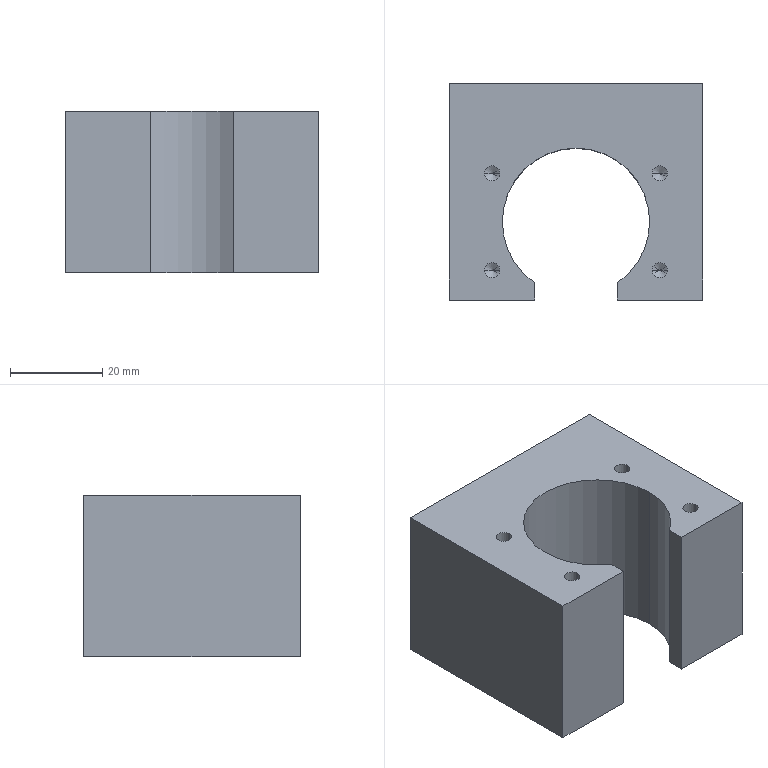Part | SolidWorks | features HoleWzd 2, 3DProfileFeature 1, Extrusion 1 | 1 solid | 52 faces | box 55 x 47 x 35 mm | volume 59809 mm3 | cone 24 | cylinder 19 | plane 9 | commonest cylinder face diameters 3.3 x8 5 x8 32 x3
STEP:
#1=CARTESIAN_POINT('',(-20.5,29.475,8.));
#2=VERTEX_POINT('',#1);
#3=CARTESIAN_POINT('',(-20.5,29.475,13.));
#4=VERTEX_POINT('',#3);
#5=CARTESIAN_POINT('',(-20.5,29.475,10.5));
#6=DIRECTION('',(0.,1.,0.));
#7=DIRECTION('',(0.,0.,1.));
#8=AXIS2_PLACEMENT_3D('',#5,#6,#7);
#9=CIRCLE('',#8,2.5);
#10=EDGE_CURVE('',#2,#4,#9,.T.);
#11=ORIENTED_EDGE('',*,*,#10,.F.);
#12=CARTESIAN_POINT('',(-20.5,30.,7.475));
#13=VERTEX_POINT('',#12);
#14=CARTESIAN_POINT('',(-20.5,30.,7.475));
#15=DIRECTION('',(0.,0.7071,-0.7071));
#16=VECTOR('',#15,1000.);
#17=LINE('',#14,#16);
#18=EDGE_CURVE('',#2,#13,#17,.T.);
#19=ORIENTED_EDGE('',*,*,#18,.T.);
#20=CARTESIAN_POINT('',(-20.5,30.,13.525));
#21=VERTEX_POINT('',#20);
#22=CARTESIAN_POINT('',(-20.5,30.,10.5));
#23=DIRECTION('',(0.,1.,0.));
#24=DIRECTION('',(0.,0.,1.));
#25=AXIS2_PLACEMENT_3D('',#22,#23,#24);
#26=CIRCLE('',#25,3.025);
#27=EDGE_CURVE('',#13,#21,#26,.T.);
#28=ORIENTED_EDGE('',*,*,#27,.T.);
#29=CARTESIAN_POINT('',(-20.5,30.,13.525));
#30=DIRECTION('',(0.,0.7071,0.7071));
#31=VECTOR('',#30,1000.);
#32=LINE('',#29,#31);
#33=EDGE_CURVE('',#4,#21,#32,.T.);
#34=ORIENTED_EDGE('',*,*,#33,.F.);
#35=EDGE_LOOP('',(#11,#19,#28,#34));
#36=FACE_OUTER_BOUND('',#35,.T.);
#37=CARTESIAN_POINT('',(-20.5,30.,10.5));
#38=DIRECTION('',(0.,1.,0.));
#39=DIRECTION('',(0.,0.,1.));
#40=AXIS2_PLACEMENT_3D('',#37,#38,#39);
#41=CONICAL_SURFACE('',#40,3.025,0.7854);
#42=ADVANCED_FACE('',(#36),#41,.F.);
#43=CARTESIAN_POINT('',(-20.5,18.,8.));
#44=VERTEX_POINT('',#43);
#45=CARTESIAN_POINT('',(-20.5,18.,13.));
#46=VERTEX_POINT('',#45);
#47=CARTESIAN_POINT('',(-20.5,18.,10.5));
#48=DIRECTION('',(0.,1.,0.));
#49=DIRECTION('',(0.,0.,1.));
#50=AXIS2_PLACEMENT_3D('',#47,#48,#49);
#51=CIRCLE('',#50,2.5);
#52=EDGE_CURVE('',#44,#46,#51,.T.);
#53=ORIENTED_EDGE('',*,*,#52,.F.);
#54=CARTESIAN_POINT('',(-20.5,30.,8.));
#55=DIRECTION('',(0.,1.,0.));
#56=VECTOR('',#55,1000.);
#57=LINE('',#54,#56);
#58=EDGE_CURVE('',#44,#2,#57,.T.);
#59=ORIENTED_EDGE('',*,*,#58,.T.);
#60=ORIENTED_EDGE('',*,*,#10,.T.);
#61=CARTESIAN_POINT('',(-20.5,30.,13.));
#62=DIRECTION('',(0.,1.,0.));
#63=VECTOR('',#62,1000.);
#64=LINE('',#61,#63);
#65=EDGE_CURVE('',#46,#4,#64,.T.);
#66=ORIENTED_EDGE('',*,*,#65,.F.);
#67=EDGE_LOOP('',(#53,#59,#60,#66));
#68=FACE_OUTER_BOUND('',#67,.T.);
#69=CARTESIAN_POINT('',(-20.5,30.,10.5));
#70=DIRECTION('',(0.,1.,0.));
#71=DIRECTION('',(0.,0.,1.));
#72=AXIS2_PLACEMENT_3D('',#69,#70,#71);
#73=CYLINDRICAL_SURFACE('',#72,2.5);
#74=ADVANCED_FACE('',(#68),#73,.F.);
#75=CARTESIAN_POINT('',(-20.5,16.498,10.5));
#76=VERTEX_POINT('',#75);
#77=CARTESIAN_POINT('',(-20.5,18.,13.));
#78=DIRECTION('',(0.,0.515,0.8572));
#79=VECTOR('',#78,1000.);
#80=LINE('',#77,#79);
#81=EDGE_CURVE('',#76,#46,#80,.T.);
#82=ORIENTED_EDGE('',*,*,#81,.F.);
#83=CARTESIAN_POINT('',(-20.5,18.,8.));
#84=DIRECTION('',(0.,0.515,-0.8572));
#85=VECTOR('',#84,1000.);
#86=LINE('',#83,#85);
#87=EDGE_CURVE('',#76,#44,#86,.T.);
#88=ORIENTED_EDGE('',*,*,#87,.T.);
#89=ORIENTED_EDGE('',*,*,#52,.T.);
#90=EDGE_LOOP('',(#82,#88,#89));
#91=FACE_OUTER_BOUND('',#90,.T.);
#92=CARTESIAN_POINT('',(-20.5,18.,10.5));
#93=DIRECTION('',(0.,1.,0.));
#94=DIRECTION('',(0.,0.,1.));
#95=AXIS2_PLACEMENT_3D('',#92,#93,#94);
#96=CONICAL_SURFACE('',#95,2.5,1.03);
#97=ADVANCED_FACE('',(#91),#96,.F.);
#98=CARTESIAN_POINT('',(-20.5,29.475,-13.));
#99=VERTEX_POINT('',#98);
#100=CARTESIAN_POINT('',(-20.5,29.475,-8.));
#101=VERTEX_POINT('',#100);
#102=CARTESIAN_POINT('',(-20.5,29.475,-10.5));
#103=DIRECTION('',(0.,1.,0.));
#104=DIRECTION('',(0.,0.,1.));
#105=AXIS2_PLACEMENT_3D('',#102,#103,#104);
#106=CIRCLE('',#105,2.5);
#107=EDGE_CURVE('',#99,#101,#106,.T.);
#108=ORIENTED_EDGE('',*,*,#107,.F.);
#109=CARTESIAN_POINT('',(-20.5,30.,-13.525));
#110=VERTEX_POINT('',#109);
#111=CARTESIAN_POINT('',(-20.5,30.,-13.525));
#112=DIRECTION('',(0.,0.7071,-0.7071));
#113=VECTOR('',#112,1000.);
#114=LINE('',#111,#113);
#115=EDGE_CURVE('',#99,#110,#114,.T.);
#116=ORIENTED_EDGE('',*,*,#115,.T.);
#117=CARTESIAN_POINT('',(-20.5,30.,-7.475));
#118=VERTEX_POINT('',#117);
#119=CARTESIAN_POINT('',(-20.5,30.,-10.5));
#120=DIRECTION('',(0.,1.,0.));
#121=DIRECTION('',(0.,0.,1.));
#122=AXIS2_PLACEMENT_3D('',#119,#120,#121);
#123=CIRCLE('',#122,3.025);
#124=EDGE_CURVE('',#110,#118,#123,.T.);
#125=ORIENTED_EDGE('',*,*,#124,.T.);
#126=CARTESIAN_POINT('',(-20.5,30.,-7.475));
#127=DIRECTION('',(0.,0.7071,0.7071));
#128=VECTOR('',#127,1000.);
#129=LINE('',#126,#128);
#130=EDGE_CURVE('',#101,#118,#129,.T.);
#131=ORIENTED_EDGE('',*,*,#130,.F.);
#132=EDGE_LOOP('',(#108,#116,#125,#131));
#133=FACE_OUTER_BOUND('',#132,.T.);
#134=CARTESIAN_POINT('',(-20.5,30.,-10.5));
#135=DIRECTION('',(0.,1.,0.));
#136=DIRECTION('',(0.,0.,1.));
#137=AXIS2_PLACEMENT_3D('',#134,#135,#136);
#138=CONICAL_SURFACE('',#137,3.025,0.7854);
#139=ADVANCED_FACE('',(#133),#138,.F.);
#140=CARTESIAN_POINT('',(-20.5,18.,-13.));
#141=VERTEX_POINT('',#140);
#142=CARTESIAN_POINT('',(-20.5,18.,-8.));
#143=VERTEX_POINT('',#142);
#144=CARTESIAN_POINT('',(-20.5,18.,-10.5));
#145=DIRECTION('',(0.,1.,0.));
#146=DIRECTION('',(0.,0.,1.));
#147=AXIS2_PLACEMENT_3D('',#144,#145,#146);
#148=CIRCLE('',#147,2.5);
#149=EDGE_CURVE('',#141,#143,#148,.T.);
#150=ORIENTED_EDGE('',*,*,#149,.F.);
#151=CARTESIAN_POINT('',(-20.5,30.,-13.));
#152=DIRECTION('',(0.,1.,0.));
#153=VECTOR('',#152,1000.);
#154=LINE('',#151,#153);
#155=EDGE_CURVE('',#141,#99,#154,.T.);
#156=ORIENTED_EDGE('',*,*,#155,.T.);
#157=ORIENTED_EDGE('',*,*,#107,.T.);
#158=CARTESIAN_POINT('',(-20.5,30.,-8.));
#159=DIRECTION('',(0.,1.,0.));
#160=VECTOR('',#159,1000.);
#161=LINE('',#158,#160);
#162=EDGE_CURVE('',#143,#101,#161,.T.);
#163=ORIENTED_EDGE('',*,*,#162,.F.);
#164=EDGE_LOOP('',(#150,#156,#157,#163));
#165=FACE_OUTER_BOUND('',#164,.T.);
#166=CARTESIAN_POINT('',(-20.5,30.,-10.5));
#167=DIRECTION('',(0.,1.,0.));
#168=DIRECTION('',(0.,0.,1.));
#169=AXIS2_PLACEMENT_3D('',#166,#167,#168);
#170=CYLINDRICAL_SURFACE('',#169,2.5);
#171=ADVANCED_FACE('',(#165),#170,.F.);
#172=CARTESIAN_POINT('',(-20.5,16.498,-10.5));
#173=VERTEX_POINT('',#172);
#174=CARTESIAN_POINT('',(-20.5,18.,-8.));
#175=DIRECTION('',(0.,0.515,0.8572));
#176=VECTOR('',#175,1000.);
#177=LINE('',#174,#176);
#178=EDGE_CURVE('',#173,#143,#177,.T.);
#179=ORIENTED_EDGE('',*,*,#178,.F.);
#180=CARTESIAN_POINT('',(-20.5,18.,-13.));
#181=DIRECTION('',(0.,0.515,-0.8572));
#182=VECTOR('',#181,1000.);
#183=LINE('',#180,#182);
#184=EDGE_CURVE('',#173,#141,#183,.T.);
#185=ORIENTED_EDGE('',*,*,#184,.T.);
#186=ORIENTED_EDGE('',*,*,#149,.T.);
#187=EDGE_LOOP('',(#179,#185,#186));
#188=FACE_OUTER_BOUND('',#187,.T.);
#189=CARTESIAN_POINT('',(-20.5,18.,-10.5));
#190=DIRECTION('',(0.,1.,0.));
#191=DIRECTION('',(0.,0.,1.));
#192=AXIS2_PLACEMENT_3D('',#189,#190,#191);
#193=CONICAL_SURFACE('',#192,2.5,1.03);
#194=ADVANCED_FACE('',(#188),#193,.F.);
#195=CARTESIAN_POINT('',(20.5,29.475,-13.));
#196=VERTEX_POINT('',#195);
#197=CARTESIAN_POINT('',(20.5,29.475,-8.));
#198=VERTEX_POINT('',#197);
#199=CARTESIAN_POINT('',(20.5,29.475,-10.5));
#200=DIRECTION('',(0.,1.,0.));
#201=DIRECTION('',(0.,0.,1.));
#202=AXIS2_PLACEMENT_3D('',#199,#200,#201);
#203=CIRCLE('',#202,2.5);
#204=EDGE_CURVE('',#196,#198,#203,.T.);
#205=ORIENTED_EDGE('',*,*,#204,.F.);
#206=CARTESIAN_POINT('',(20.5,30.,-13.525));
#207=VERTEX_POINT('',#206);
#208=CARTESIAN_POINT('',(20.5,30.,-13.525));
#209=DIRECTION('',(0.,0.7071,-0.7071));
#210=VECTOR('',#209,1000.);
#211=LINE('',#208,#210);
#212=EDGE_CURVE('',#196,#207,#211,.T.);
#213=ORIENTED_EDGE('',*,*,#212,.T.);
#214=CARTESIAN_POINT('',(20.5,30.,-7.475));
#215=VERTEX_POINT('',#214);
#216=CARTESIAN_POINT('',(20.5,30.,-10.5));
#217=DIRECTION('',(0.,1.,0.));
#218=DIRECTION('',(0.,0.,1.));
#219=AXIS2_PLACEMENT_3D('',#216,#217,#218);
#220=CIRCLE('',#219,3.025);
#221=EDGE_CURVE('',#207,#215,#220,.T.);
#222=ORIENTED_EDGE('',*,*,#221,.T.);
#223=CARTESIAN_POINT('',(20.5,30.,-7.475));
#224=DIRECTION('',(0.,0.7071,0.7071));
#225=VECTOR('',#224,1000.);
#226=LINE('',#223,#225);
#227=EDGE_CURVE('',#198,#215,#226,.T.);
#228=ORIENTED_EDGE('',*,*,#227,.F.);
#229=EDGE_LOOP('',(#205,#213,#222,#228));
#230=FACE_OUTER_BOUND('',#229,.T.);
#231=CARTESIAN_POINT('',(20.5,30.,-10.5));
#232=DIRECTION('',(0.,1.,0.));
#233=DIRECTION('',(0.,0.,1.));
#234=AXIS2_PLACEMENT_3D('',#231,#232,#233);
#235=CONICAL_SURFACE('',#234,3.025,0.7854);
#236=ADVANCED_FACE('',(#230),#235,.F.);
#237=CARTESIAN_POINT('',(20.5,18.,-13.));
#238=VERTEX_POINT('',#237);
#239=CARTESIAN_POINT('',(20.5,18.,-8.));
#240=VERTEX_POINT('',#239);
#241=CARTESIAN_POINT('',(20.5,18.,-10.5));
#242=DIRECTION('',(0.,1.,0.));
#243=DIRECTION('',(0.,0.,1.));
#244=AXIS2_PLACEMENT_3D('',#241,#242,#243);
#245=CIRCLE('',#244,2.5);
#246=EDGE_CURVE('',#238,#240,#245,.T.);
#247=ORIENTED_EDGE('',*,*,#246,.F.);
#248=CARTESIAN_POINT('',(20.5,30.,-13.));
#249=DIRECTION('',(0.,1.,0.));
#250=VECTOR('',#249,1000.);
#251=LINE('',#248,#250);
#252=EDGE_CURVE('',#238,#196,#251,.T.);
#253=ORIENTED_EDGE('',*,*,#252,.T.);
#254=ORIENTED_EDGE('',*,*,#204,.T.);
#255=CARTESIAN_POINT('',(20.5,30.,-8.));
#256=DIRECTION('',(0.,1.,0.));
#257=VECTOR('',#256,1000.);
#258=LINE('',#255,#257);
#259=EDGE_CURVE('',#240,#198,#258,.T.);
#260=ORIENTED_EDGE('',*,*,#259,.F.);
#261=EDGE_LOOP('',(#247,#253,#254,#260));
#262=FACE_OUTER_BOUND('',#261,.T.);
#263=CARTESIAN_POINT('',(20.5,30.,-10.5));
#264=DIRECTION('',(0.,1.,0.));
#265=DIRECTION('',(0.,0.,1.));
#266=AXIS2_PLACEMENT_3D('',#263,#264,#265);
#267=CYLINDRICAL_SURFACE('',#266,2.5);
#268=ADVANCED_FACE('',(#262),#267,.F.);
#269=CARTESIAN_POINT('',(20.5,16.498,-10.5));
#270=VERTEX_POINT('',#269);
#271=CARTESIAN_POINT('',(20.5,18.,-8.));
#272=DIRECTION('',(0.,0.515,0.8572));
#273=VECTOR('',#272,1000.);
#274=LINE('',#271,#273);
#275=EDGE_CURVE('',#270,#240,#274,.T.);
#276=ORIENTED_EDGE('',*,*,#275,.F.);
#277=CARTESIAN_POINT('',(20.5,18.,-13.));
#278=DIRECTION('',(0.,0.515,-0.8572));
#279=VECTOR('',#278,1000.);
#280=LINE('',#277,#279);
#281=EDGE_CURVE('',#270,#238,#280,.T.);
#282=ORIENTED_EDGE('',*,*,#281,.T.);
#283=ORIENTED_EDGE('',*,*,#246,.T.);
#284=EDGE_LOOP('',(#276,#282,#283));
#285=FACE_OUTER_BOUND('',#284,.T.);
#286=CARTESIAN_POINT('',(20.5,18.,-10.5));
#287=DIRECTION('',(0.,1.,0.));
#288=DIRECTION('',(0.,0.,1.));
#289=AXIS2_PLACEMENT_3D('',#286,#287,#288);
#290=CONICAL_SURFACE('',#289,2.5,1.03);
#291=ADVANCED_FACE('',(#285),#290,.F.);
#292=CARTESIAN_POINT('',(20.5,29.475,8.));
#293=VERTEX_POINT('',#292);
#294=CARTESIAN_POINT('',(20.5,29.475,13.));
#295=VERTEX_POINT('',#294);
#296=CARTESIAN_POINT('',(20.5,29.475,10.5));
#297=DIRECTION('',(0.,1.,0.));
#298=DIRECTION('',(0.,0.,1.));
#299=AXIS2_PLACEMENT_3D('',#296,#297,#298);
#300=CIRCLE('',#299,2.5);
#301=EDGE_CURVE('',#293,#295,#300,.T.);
#302=ORIENTED_EDGE('',*,*,#301,.F.);
#303=CARTESIAN_POINT('',(20.5,30.,7.475));
#304=VERTEX_POINT('',#303);
#305=CARTESIAN_POINT('',(20.5,30.,7.475));
#306=DIRECTION('',(0.,0.7071,-0.7071));
#307=VECTOR('',#306,1000.);
#308=LINE('',#305,#307);
#309=EDGE_CURVE('',#293,#304,#308,.T.);
#310=ORIENTED_EDGE('',*,*,#309,.T.);
#311=CARTESIAN_POINT('',(20.5,30.,13.525));
#312=VERTEX_POINT('',#311);
#313=CARTESIAN_POINT('',(20.5,30.,10.5));
#314=DIRECTION('',(0.,1.,0.));
#315=DIRECTION('',(0.,0.,1.));
#316=AXIS2_PLACEMENT_3D('',#313,#314,#315);
#317=CIRCLE('',#316,3.025);
#318=EDGE_CURVE('',#304,#312,#317,.T.);
#319=ORIENTED_EDGE('',*,*,#318,.T.);
#320=CARTESIAN_POINT('',(20.5,30.,13.525));
#321=DIRECTION('',(0.,0.7071,0.7071));
#322=VECTOR('',#321,1000.);
#323=LINE('',#320,#322);
#324=EDGE_CURVE('',#295,#312,#323,.T.);
#325=ORIENTED_EDGE('',*,*,#324,.F.);
#326=EDGE_LOOP('',(#302,#310,#319,#325));
#327=FACE_OUTER_BOUND('',#326,.T.);
#328=CARTESIAN_POINT('',(20.5,30.,10.5));
#329=DIRECTION('',(0.,1.,0.));
#330=DIRECTION('',(0.,0.,1.));
#331=AXIS2_PLACEMENT_3D('',#328,#329,#330);
#332=CONICAL_SURFACE('',#331,3.025,0.7854);
#333=ADVANCED_FACE('',(#327),#332,.F.);
#334=CARTESIAN_POINT('',(20.5,18.,8.));
#335=VERTEX_POINT('',#334);
#336=CARTESIAN_POINT('',(20.5,18.,13.));
#337=VERTEX_POINT('',#336);
#338=CARTESIAN_POINT('',(20.5,18.,10.5));
#339=DIRECTION('',(0.,1.,0.));
#340=DIRECTION('',(0.,0.,1.));
#341=AXIS2_PLACEMENT_3D('',#338,#339,#340);
#342=CIRCLE('',#341,2.5);
#343=EDGE_CURVE('',#335,#337,#342,.T.);
#344=ORIENTED_EDGE('',*,*,#343,.F.);
#345=CARTESIAN_POINT('',(20.5,30.,8.));
#346=DIRECTION('',(0.,1.,0.));
#347=VECTOR('',#346,1000.);
#348=LINE('',#345,#347);
#349=EDGE_CURVE('',#335,#293,#348,.T.);
#350=ORIENTED_EDGE('',*,*,#349,.T.);
#351=ORIENTED_EDGE('',*,*,#301,.T.);
#352=CARTESIAN_POINT('',(20.5,30.,13.));
#353=DIRECTION('',(0.,1.,0.));
#354=VECTOR('',#353,1000.);
#355=LINE('',#352,#354);
#356=EDGE_CURVE('',#337,#295,#355,.T.);
#357=ORIENTED_EDGE('',*,*,#356,.F.);
#358=EDGE_LOOP('',(#344,#350,#351,#357));
#359=FACE_OUTER_BOUND('',#358,.T.);
#360=CARTESIAN_POINT('',(20.5,30.,10.5));
#361=DIRECTION('',(0.,1.,0.));
#362=DIRECTION('',(0.,0.,1.));
#363=AXIS2_PLACEMENT_3D('',#360,#361,#362);
#364=CYLINDRICAL_SURFACE('',#363,2.5);
#365=ADVANCED_FACE('',(#359),#364,.F.);
#366=CARTESIAN_POINT('',(20.5,16.498,10.5));
#367=VERTEX_POINT('',#366);
#368=CARTESIAN_POINT('',(20.5,18.,13.));
#369=DIRECTION('',(0.,0.515,0.8572));
#370=VECTOR('',#369,1000.);
#371=LINE('',#368,#370);
#372=EDGE_CURVE('',#367,#337,#371,.T.);
#373=ORIENTED_EDGE('',*,*,#372,.F.);
#374=CARTESIAN_POINT('',(20.5,18.,8.));
#375=DIRECTION('',(0.,0.515,-0.8572));
#376=VECTOR('',#375,1000.);
#377=LINE('',#374,#376);
#378=EDGE_CURVE('',#367,#335,#377,.T.);
#379=ORIENTED_EDGE('',*,*,#378,.T.);
#380=ORIENTED_EDGE('',*,*,#343,.T.);
#381=EDGE_LOOP('',(#373,#379,#380));
#382=FACE_OUTER_BOUND('',#381,.T.);
#383=CARTESIAN_POINT('',(20.5,18.,10.5));
#384=DIRECTION('',(0.,1.,0.));
#385=DIRECTION('',(0.,0.,1.));
#386=AXIS2_PLACEMENT_3D('',#383,#384,#385);
#387=CONICAL_SURFACE('',#386,2.5,1.03);
#388=ADVANCED_FACE('',(#382),#387,.F.);
#389=CARTESIAN_POINT('',(16.537,10.5,8.));
#390=VERTEX_POINT('',#389);
#391=CARTESIAN_POINT('',(19.837,10.5,8.));
#392=VERTEX_POINT('',#391);
#393=CARTESIAN_POINT('',(18.187,10.5,8.));
#394=DIRECTION('',(0.,0.,1.));
#395=DIRECTION('',(1.,0.,0.));
#396=AXIS2_PLACEMENT_3D('',#393,#394,#395);
#397=CIRCLE('',#396,1.65);
#398=EDGE_CURVE('',#390,#392,#397,.T.);
#399=ORIENTED_EDGE('',*,*,#398,.F.);
#400=CARTESIAN_POINT('',(16.537,10.5,17.5));
#401=VERTEX_POINT('',#400);
#402=CARTESIAN_POINT('',(16.537,10.5,17.5));
#403=DIRECTION('',(0.,0.,1.));
#404=VECTOR('',#403,1000.);
#405=LINE('',#402,#404);
#406=EDGE_CURVE('',#390,#401,#405,.T.);
#407=ORIENTED_EDGE('',*,*,#406,.T.);
#408=CARTESIAN_POINT('',(19.837,10.5,17.5));
#409=VERTEX_POINT('',#408);
#410=CARTESIAN_POINT('',(18.187,10.5,17.5));
#411=DIRECTION('',(0.,0.,1.));
#412=DIRECTION('',(1.,0.,0.));
#413=AXIS2_PLACEMENT_3D('',#410,#411,#412);
#414=CIRCLE('',#413,1.65);
#415=EDGE_CURVE('',#401,#409,#414,.T.);
#416=ORIENTED_EDGE('',*,*,#415,.T.);
#417=CARTESIAN_POINT('',(19.837,10.5,17.5));
#418=DIRECTION('',(0.,0.,1.));
#419=VECTOR('',#418,1000.);
#420=LINE('',#417,#419);
#421=EDGE_CURVE('',#392,#409,#420,.T.);
#422=ORIENTED_EDGE('',*,*,#421,.F.);
#423=EDGE_LOOP('',(#399,#407,#416,#422));
#424=FACE_OUTER_BOUND('',#423,.T.);
#425=CARTESIAN_POINT('',(18.187,10.5,17.5));
#426=DIRECTION('',(0.,0.,1.));
#427=DIRECTION('',(1.,0.,0.));
#428=AXIS2_PLACEMENT_3D('',#425,#426,#427);
#429=CYLINDRICAL_SURFACE('',#428,1.65);
#430=ADVANCED_FACE('',(#424),#429,.F.);
#431=CARTESIAN_POINT('',(18.187,10.5,7.009));
#432=VERTEX_POINT('',#431);
#433=CARTESIAN_POINT('',(19.837,10.5,8.));
#434=DIRECTION('',(0.8572,0.,0.515));
#435=VECTOR('',#434,1000.);
#436=LINE('',#433,#435);
#437=EDGE_CURVE('',#432,#392,#436,.T.);
#438=ORIENTED_EDGE('',*,*,#437,.F.);
#439=CARTESIAN_POINT('',(16.537,10.5,8.));
#440=DIRECTION('',(-0.8572,0.,0.515));
#441=VECTOR('',#440,1000.);
#442=LINE('',#439,#441);
#443=EDGE_CURVE('',#432,#390,#442,.T.);
#444=ORIENTED_EDGE('',*,*,#443,.T.);
#445=ORIENTED_EDGE('',*,*,#398,.T.);
#446=EDGE_LOOP('',(#438,#444,#445));
#447=FACE_OUTER_BOUND('',#446,.T.);
#448=CARTESIAN_POINT('',(18.187,10.5,8.));
#449=DIRECTION('',(0.,0.,1.));
#450=DIRECTION('',(1.,0.,0.));
#451=AXIS2_PLACEMENT_3D('',#448,#449,#450);
#452=CONICAL_SURFACE('',#451,1.65,1.03);
#453=ADVANCED_FACE('',(#447),#452,.F.);
#454=CARTESIAN_POINT('',(16.537,-10.5,8.));
#455=VERTEX_POINT('',#454);
#456=CARTESIAN_POINT('',(19.837,-10.5,8.));
#457=VERTEX_POINT('',#456);
#458=CARTESIAN_POINT('',(18.187,-10.5,8.));
#459=DIRECTION('',(0.,0.,1.));
#460=DIRECTION('',(1.,0.,0.));
#461=AXIS2_PLACEMENT_3D('',#458,#459,#460);
#462=CIRCLE('',#461,1.65);
#463=EDGE_CURVE('',#455,#457,#462,.T.);
#464=ORIENTED_EDGE('',*,*,#463,.F.);
#465=CARTESIAN_POINT('',(16.537,-10.5,17.5));
#466=VERTEX_POINT('',#465);
#467=CARTESIAN_POINT('',(16.537,-10.5,17.5));
#468=DIRECTION('',(0.,0.,1.));
#469=VECTOR('',#468,1000.);
#470=LINE('',#467,#469);
#471=EDGE_CURVE('',#455,#466,#470,.T.);
#472=ORIENTED_EDGE('',*,*,#471,.T.);
#473=CARTESIAN_POINT('',(19.837,-10.5,17.5));
#474=VERTEX_POINT('',#473);
#475=CARTESIAN_POINT('',(18.187,-10.5,17.5));
#476=DIRECTION('',(0.,0.,1.));
#477=DIRECTION('',(1.,0.,0.));
#478=AXIS2_PLACEMENT_3D('',#475,#476,#477);
#479=CIRCLE('',#478,1.65);
#480=EDGE_CURVE('',#466,#474,#479,.T.);
#481=ORIENTED_EDGE('',*,*,#480,.T.);
#482=CARTESIAN_POINT('',(19.837,-10.5,17.5));
#483=DIRECTION('',(0.,0.,1.));
#484=VECTOR('',#483,1000.);
#485=LINE('',#482,#484);
#486=EDGE_CURVE('',#457,#474,#485,.T.);
#487=ORIENTED_EDGE('',*,*,#486,.F.);
#488=EDGE_LOOP('',(#464,#472,#481,#487));
#489=FACE_OUTER_BOUND('',#488,.T.);
#490=CARTESIAN_POINT('',(18.187,-10.5,17.5));
#491=DIRECTION('',(0.,0.,1.));
#492=DIRECTION('',(1.,0.,0.));
#493=AXIS2_PLACEMENT_3D('',#490,#491,#492);
#494=CYLINDRICAL_SURFACE('',#493,1.65);
#495=ADVANCED_FACE('',(#489),#494,.F.);
#496=CARTESIAN_POINT('',(18.187,-10.5,7.009));
#497=VERTEX_POINT('',#496);
#498=CARTESIAN_POINT('',(19.837,-10.5,8.));
#499=DIRECTION('',(0.8572,0.,0.515));
#500=VECTOR('',#499,1000.);
#501=LINE('',#498,#500);
#502=EDGE_CURVE('',#497,#457,#501,.T.);
#503=ORIENTED_EDGE('',*,*,#502,.F.);
#504=CARTESIAN_POINT('',(16.537,-10.5,8.));
#505=DIRECTION('',(-0.8572,0.,0.515));
#506=VECTOR('',#505,1000.);
#507=LINE('',#504,#506);
#508=EDGE_CURVE('',#497,#455,#507,.T.);
#509=ORIENTED_EDGE('',*,*,#508,.T.);
#510=ORIENTED_EDGE('',*,*,#463,.T.);
#511=EDGE_LOOP('',(#503,#509,#510));
#512=FACE_OUTER_BOUND('',#511,.T.);
#513=CARTESIAN_POINT('',(18.187,-10.5,8.));
#514=DIRECTION('',(0.,0.,1.));
#515=DIRECTION('',(1.,0.,0.));
#516=AXIS2_PLACEMENT_3D('',#513,#514,#515);
#517=CONICAL_SURFACE('',#516,1.65,1.03);
#518=ADVANCED_FACE('',(#512),#517,.F.);
#519=CARTESIAN_POINT('',(-19.837,-10.5,8.));
#520=VERTEX_POINT('',#519);
#521=CARTESIAN_POINT('',(-16.537,-10.5,8.));
#522=VERTEX_POINT('',#521);
#523=CARTESIAN_POINT('',(-18.187,-10.5,8.));
#524=DIRECTION('',(0.,0.,1.));
#525=DIRECTION('',(1.,0.,0.));
#526=AXIS2_PLACEMENT_3D('',#523,#524,#525);
#527=CIRCLE('',#526,1.65);
#528=EDGE_CURVE('',#520,#522,#527,.T.);
#529=ORIENTED_EDGE('',*,*,#528,.F.);
#530=CARTESIAN_POINT('',(-19.837,-10.5,17.5));
#531=VERTEX_POINT('',#530);
#532=CARTESIAN_POINT('',(-19.837,-10.5,17.5));
#533=DIRECTION('',(0.,0.,1.));
#534=VECTOR('',#533,1000.);
#535=LINE('',#532,#534);
#536=EDGE_CURVE('',#520,#531,#535,.T.);
#537=ORIENTED_EDGE('',*,*,#536,.T.);
#538=CARTESIAN_POINT('',(-16.537,-10.5,17.5));
#539=VERTEX_POINT('',#538);
#540=CARTESIAN_POINT('',(-18.187,-10.5,17.5));
#541=DIRECTION('',(0.,0.,1.));
#542=DIRECTION('',(1.,0.,0.));
#543=AXIS2_PLACEMENT_3D('',#540,#541,#542);
#544=CIRCLE('',#543,1.65);
#545=EDGE_CURVE('',#531,#539,#544,.T.);
#546=ORIENTED_EDGE('',*,*,#545,.T.);
#547=CARTESIAN_POINT('',(-16.537,-10.5,17.5));
#548=DIRECTION('',(0.,0.,1.));
#549=VECTOR('',#548,1000.);
#550=LINE('',#547,#549);
#551=EDGE_CURVE('',#522,#539,#550,.T.);
#552=ORIENTED_EDGE('',*,*,#551,.F.);
#553=EDGE_LOOP('',(#529,#537,#546,#552));
#554=FACE_OUTER_BOUND('',#553,.T.);
#555=CARTESIAN_POINT('',(-18.187,-10.5,17.5));
#556=DIRECTION('',(0.,0.,1.));
#557=DIRECTION('',(1.,0.,0.));
#558=AXIS2_PLACEMENT_3D('',#555,#556,#557);
#559=CYLINDRICAL_SURFACE('',#558,1.65);
#560=ADVANCED_FACE('',(#554),#559,.F.);
#561=CARTESIAN_POINT('',(-18.187,-10.5,7.009));
#562=VERTEX_POINT('',#561);
#563=CARTESIAN_POINT('',(-16.537,-10.5,8.));
#564=DIRECTION('',(0.8572,0.,0.515));
#565=VECTOR('',#564,1000.);
#566=LINE('',#563,#565);
#567=EDGE_CURVE('',#562,#522,#566,.T.);
#568=ORIENTED_EDGE('',*,*,#567,.F.);
#569=CARTESIAN_POINT('',(-19.837,-10.5,8.));
#570=DIRECTION('',(-0.8572,0.,0.515));
#571=VECTOR('',#570,1000.);
#572=LINE('',#569,#571);
#573=EDGE_CURVE('',#562,#520,#572,.T.);
#574=ORIENTED_EDGE('',*,*,#573,.T.);
#575=ORIENTED_EDGE('',*,*,#528,.T.);
#576=EDGE_LOOP('',(#568,#574,#575));
#577=FACE_OUTER_BOUND('',#576,.T.);
#578=CARTESIAN_POINT('',(-18.187,-10.5,8.));
#579=DIRECTION('',(0.,0.,1.));
#580=DIRECTION('',(1.,0.,0.));
#581=AXIS2_PLACEMENT_3D('',#578,#579,#580);
#582=CONICAL_SURFACE('',#581,1.65,1.03);
#583=ADVANCED_FACE('',(#577),#582,.F.);
#584=CARTESIAN_POINT('',(-19.837,10.5,8.));
#585=VERTEX_POINT('',#584);
#586=CARTESIAN_POINT('',(-16.537,10.5,8.));
#587=VERTEX_POINT('',#586);
#588=CARTESIAN_POINT('',(-18.187,10.5,8.));
#589=DIRECTION('',(0.,0.,1.));
#590=DIRECTION('',(1.,0.,0.));
#591=AXIS2_PLACEMENT_3D('',#588,#589,#590);
#592=CIRCLE('',#591,1.65);
#593=EDGE_CURVE('',#585,#587,#592,.T.);
#594=ORIENTED_EDGE('',*,*,#593,.F.);
#595=CARTESIAN_POINT('',(-19.837,10.5,17.5));
#596=VERTEX_POINT('',#595);
#597=CARTESIAN_POINT('',(-19.837,10.5,17.5));
#598=DIRECTION('',(0.,0.,1.));
#599=VECTOR('',#598,1000.);
#600=LINE('',#597,#599);
#601=EDGE_CURVE('',#585,#596,#600,.T.);
#602=ORIENTED_EDGE('',*,*,#601,.T.);
#603=CARTESIAN_POINT('',(-16.537,10.5,17.5));
#604=VERTEX_POINT('',#603);
#605=CARTESIAN_POINT('',(-18.187,10.5,17.5));
#606=DIRECTION('',(0.,0.,1.));
#607=DIRECTION('',(1.,0.,0.));
#608=AXIS2_PLACEMENT_3D('',#605,#606,#607);
#609=CIRCLE('',#608,1.65);
#610=EDGE_CURVE('',#596,#604,#609,.T.);
#611=ORIENTED_EDGE('',*,*,#610,.T.);
#612=CARTESIAN_POINT('',(-16.537,10.5,17.5));
#613=DIRECTION('',(0.,0.,1.));
#614=VECTOR('',#613,1000.);
#615=LINE('',#612,#614);
#616=EDGE_CURVE('',#587,#604,#615,.T.);
#617=ORIENTED_EDGE('',*,*,#616,.F.);
#618=EDGE_LOOP('',(#594,#602,#611,#617));
#619=FACE_OUTER_BOUND('',#618,.T.);
#620=CARTESIAN_POINT('',(-18.187,10.5,17.5));
#621=DIRECTION('',(0.,0.,1.));
#622=DIRECTION('',(1.,0.,0.));
#623=AXIS2_PLACEMENT_3D('',#620,#621,#622);
#624=CYLINDRICAL_SURFACE('',#623,1.65);
#625=ADVANCED_FACE('',(#619),#624,.F.);
#626=CARTESIAN_POINT('',(-18.187,10.5,7.009));
#627=VERTEX_POINT('',#626);
#628=CARTESIAN_POINT('',(-16.537,10.5,8.));
#629=DIRECTION('',(0.8572,0.,0.515));
#630=VECTOR('',#629,1000.);
#631=LINE('',#628,#630);
#632=EDGE_CURVE('',#627,#587,#631,.T.);
#633=ORIENTED_EDGE('',*,*,#632,.F.);
#634=CARTESIAN_POINT('',(-19.837,10.5,8.));
#635=DIRECTION('',(-0.8572,0.,0.515));
#636=VECTOR('',#635,1000.);
#637=LINE('',#634,#636);
#638=EDGE_CURVE('',#627,#585,#637,.T.);
#639=ORIENTED_EDGE('',*,*,#638,.T.);
#640=ORIENTED_EDGE('',*,*,#593,.T.);
#641=EDGE_LOOP('',(#633,#639,#640));
#642=FACE_OUTER_BOUND('',#641,.T.);
#643=CARTESIAN_POINT('',(-18.187,10.5,8.));
#644=DIRECTION('',(0.,0.,1.));
#645=DIRECTION('',(1.,0.,0.));
#646=AXIS2_PLACEMENT_3D('',#643,#644,#645);
#647=CONICAL_SURFACE('',#646,1.65,1.03);
#648=ADVANCED_FACE('',(#642),#647,.F.);
#649=CARTESIAN_POINT('',(16.,0.,17.5));
#650=VERTEX_POINT('',#649);
#651=CARTESIAN_POINT('',(9.,-13.229,17.5));
#652=VERTEX_POINT('',#651);
#653=CARTESIAN_POINT('',(0.,0.,17.5));
#654=DIRECTION('',(0.,0.,-1.));
#655=DIRECTION('',(1.,0.,0.));
#656=AXIS2_PLACEMENT_3D('',#653,#654,#655);
#657=CIRCLE('',#656,16.);
#658=EDGE_CURVE('',#650,#652,#657,.T.);
#659=ORIENTED_EDGE('',*,*,#658,.F.);
#660=CARTESIAN_POINT('',(16.,0.,-17.5));
#661=VERTEX_POINT('',#660);
#662=CARTESIAN_POINT('',(16.,0.,17.5));
#663=DIRECTION('',(0.,0.,-1.));
#664=VECTOR('',#663,1000.);
#665=LINE('',#662,#664);
#666=EDGE_CURVE('',#650,#661,#665,.T.);
#667=ORIENTED_EDGE('',*,*,#666,.T.);
#668=CARTESIAN_POINT('',(9.,-13.229,-17.5));
#669=VERTEX_POINT('',#668);
#670=CARTESIAN_POINT('',(0.,0.,-17.5));
#671=DIRECTION('',(0.,0.,-1.));
#672=DIRECTION('',(1.,0.,0.));
#673=AXIS2_PLACEMENT_3D('',#670,#671,#672);
#674=CIRCLE('',#673,16.);
#675=EDGE_CURVE('',#661,#669,#674,.T.);
#676=ORIENTED_EDGE('',*,*,#675,.T.);
#677=CARTESIAN_POINT('',(9.,-13.229,17.5));
#678=DIRECTION('',(0.,0.,-1.));
#679=VECTOR('',#678,1000.);
#680=LINE('',#677,#679);
#681=EDGE_CURVE('',#652,#669,#680,.T.);
#682=ORIENTED_EDGE('',*,*,#681,.F.);
#683=EDGE_LOOP('',(#659,#667,#676,#682));
#684=FACE_OUTER_BOUND('',#683,.T.);
#685=CARTESIAN_POINT('',(0.,0.,17.5));
#686=DIRECTION('',(0.,0.,-1.));
#687=DIRECTION('',(-1.,0.,0.));
#688=AXIS2_PLACEMENT_3D('',#685,#686,#687);
#689=CYLINDRICAL_SURFACE('',#688,16.);
#690=ADVANCED_FACE('',(#684),#689,.F.);
#691=ORIENTED_EDGE('',*,*,#666,.F.);
#692=CARTESIAN_POINT('',(-16.,0.,17.5));
#693=VERTEX_POINT('',#692);
#694=CARTESIAN_POINT('',(0.,0.,17.5));
#695=DIRECTION('',(0.,0.,-1.));
#696=DIRECTION('',(1.,0.,0.));
#697=AXIS2_PLACEMENT_3D('',#694,#695,#696);
#698=CIRCLE('',#697,16.);
#699=EDGE_CURVE('',#693,#650,#698,.T.);
#700=ORIENTED_EDGE('',*,*,#699,.F.);
#701=CARTESIAN_POINT('',(-16.,0.,-17.5));
#702=VERTEX_POINT('',#701);
#703=CARTESIAN_POINT('',(-16.,0.,17.5));
#704=DIRECTION('',(0.,0.,-1.));
#705=VECTOR('',#704,1000.);
#706=LINE('',#703,#705);
#707=EDGE_CURVE('',#693,#702,#706,.T.);
#708=ORIENTED_EDGE('',*,*,#707,.T.);
#709=CARTESIAN_POINT('',(0.,0.,-17.5));
#710=DIRECTION('',(0.,0.,-1.));
#711=DIRECTION('',(1.,0.,0.));
#712=AXIS2_PLACEMENT_3D('',#709,#710,#711);
#713=CIRCLE('',#712,16.);
#714=EDGE_CURVE('',#702,#661,#713,.T.);
#715=ORIENTED_EDGE('',*,*,#714,.T.);
#716=EDGE_LOOP('',(#691,#700,#708,#715));
#717=FACE_OUTER_BOUND('',#716,.T.);
#718=CARTESIAN_POINT('',(0.,0.,17.5));
#719=DIRECTION('',(0.,0.,-1.));
#720=DIRECTION('',(-1.,0.,0.));
#721=AXIS2_PLACEMENT_3D('',#718,#719,#720);
#722=CYLINDRICAL_SURFACE('',#721,16.);
#723=ADVANCED_FACE('',(#717),#722,.F.);
#724=CARTESIAN_POINT('',(-27.5,30.,-17.5));
#725=VERTEX_POINT('',#724);
#726=CARTESIAN_POINT('',(-27.5,-17.,-17.5));
#727=VERTEX_POINT('',#726);
#728=CARTESIAN_POINT('',(-27.5,30.,-17.5));
#729=DIRECTION('',(0.,-1.,0.));
#730=VECTOR('',#729,1000.);
#731=LINE('',#728,#730);
#732=EDGE_CURVE('',#725,#727,#731,.T.);
#733=ORIENTED_EDGE('',*,*,#732,.T.);
#734=CARTESIAN_POINT('',(-27.5,-17.,17.5));
#735=VERTEX_POINT('',#734);
#736=CARTESIAN_POINT('',(-27.5,-17.,17.5));
#737=DIRECTION('',(0.,0.,-1.));
#738=VECTOR('',#737,1000.);
#739=LINE('',#736,#738);
#740=EDGE_CURVE('',#735,#727,#739,.T.);
#741=ORIENTED_EDGE('',*,*,#740,.F.);
#742=CARTESIAN_POINT('',(-27.5,30.,17.5));
#743=VERTEX_POINT('',#742);
#744=CARTESIAN_POINT('',(-27.5,30.,17.5));
#745=DIRECTION('',(0.,-1.,0.));
#746=VECTOR('',#745,1000.);
#747=LINE('',#744,#746);
#748=EDGE_CURVE('',#743,#735,#747,.T.);
#749=ORIENTED_EDGE('',*,*,#748,.F.);
#750=CARTESIAN_POINT('',(-27.5,30.,17.5));
#751=DIRECTION('',(0.,0.,-1.));
#752=VECTOR('',#751,1000.);
#753=LINE('',#750,#752);
#754=EDGE_CURVE('',#743,#725,#753,.T.);
#755=ORIENTED_EDGE('',*,*,#754,.T.);
#756=EDGE_LOOP('',(#733,#741,#749,#755));
#757=FACE_OUTER_BOUND('',#756,.T.);
#758=CARTESIAN_POINT('',(-27.5,30.,17.5));
#759=DIRECTION('',(1.,0.,0.));
#760=DIRECTION('',(0.,0.,-1.));
#761=AXIS2_PLACEMENT_3D('',#758,#759,#760);
#762=PLANE('',#761);
#763=ADVANCED_FACE('',(#757),#762,.F.);
#764=CARTESIAN_POINT('',(-9.,-17.,-17.5));
#765=VERTEX_POINT('',#764);
#766=CARTESIAN_POINT('',(-27.5,-17.,-17.5));
#767=DIRECTION('',(1.,0.,0.));
#768=VECTOR('',#767,1000.);
#769=LINE('',#766,#768);
#770=EDGE_CURVE('',#727,#765,#769,.T.);
#771=ORIENTED_EDGE('',*,*,#770,.T.);
#772=CARTESIAN_POINT('',(-9.,-17.,17.5));
#773=VERTEX_POINT('',#772);
#774=CARTESIAN_POINT('',(-9.,-17.,17.5));
#775=DIRECTION('',(0.,0.,-1.));
#776=VECTOR('',#775,1000.);
#777=LINE('',#774,#776);
#778=EDGE_CURVE('',#773,#765,#777,.T.);
#779=ORIENTED_EDGE('',*,*,#778,.F.);
#780=CARTESIAN_POINT('',(-27.5,-17.,17.5));
#781=DIRECTION('',(1.,0.,0.));
#782=VECTOR('',#781,1000.);
#783=LINE('',#780,#782);
#784=EDGE_CURVE('',#735,#773,#783,.T.);
#785=ORIENTED_EDGE('',*,*,#784,.F.);
#786=ORIENTED_EDGE('',*,*,#740,.T.);
#787=EDGE_LOOP('',(#771,#779,#785,#786));
#788=FACE_OUTER_BOUND('',#787,.T.);
#789=CARTESIAN_POINT('',(-27.5,-17.,17.5));
#790=DIRECTION('',(0.,1.,0.));
#791=DIRECTION('',(0.,0.,1.));
#792=AXIS2_PLACEMENT_3D('',#789,#790,#791);
#793=PLANE('',#792);
#794=ADVANCED_FACE('',(#788),#793,.F.);
#795=CARTESIAN_POINT('',(-9.,-13.229,-17.5));
#796=VERTEX_POINT('',#795);
#797=CARTESIAN_POINT('',(-9.,-17.,-17.5));
#798=DIRECTION('',(0.,1.,0.));
#799=VECTOR('',#798,1000.);
#800=LINE('',#797,#799);
#801=EDGE_CURVE('',#765,#796,#800,.T.);
#802=ORIENTED_EDGE('',*,*,#801,.T.);
#803=CARTESIAN_POINT('',(-9.,-13.229,17.5));
#804=VERTEX_POINT('',#803);
#805=CARTESIAN_POINT('',(-9.,-13.229,17.5));
#806=DIRECTION('',(0.,0.,-1.));
#807=VECTOR('',#806,1000.);
#808=LINE('',#805,#807);
#809=EDGE_CURVE('',#804,#796,#808,.T.);
#810=ORIENTED_EDGE('',*,*,#809,.F.);
#811=CARTESIAN_POINT('',(-9.,-17.,17.5));
#812=DIRECTION('',(0.,1.,0.));
#813=VECTOR('',#812,1000.);
#814=LINE('',#811,#813);
#815=EDGE_CURVE('',#773,#804,#814,.T.);
#816=ORIENTED_EDGE('',*,*,#815,.F.);
#817=ORIENTED_EDGE('',*,*,#778,.T.);
#818=EDGE_LOOP('',(#802,#810,#816,#817));
#819=FACE_OUTER_BOUND('',#818,.T.);
#820=CARTESIAN_POINT('',(-9.,-17.,17.5));
#821=DIRECTION('',(-1.,0.,0.));
#822=DIRECTION('',(0.,-1.,0.));
#823=AXIS2_PLACEMENT_3D('',#820,#821,#822);
#824=PLANE('',#823);
#825=ADVANCED_FACE('',(#819),#824,.F.);
#826=ORIENTED_EDGE('',*,*,#707,.F.);
#827=CARTESIAN_POINT('',(0.,0.,17.5));
#828=DIRECTION('',(0.,0.,-1.));
#829=DIRECTION('',(1.,0.,0.));
#830=AXIS2_PLACEMENT_3D('',#827,#828,#829);
#831=CIRCLE('',#830,16.);
#832=EDGE_CURVE('',#804,#693,#831,.T.);
#833=ORIENTED_EDGE('',*,*,#832,.F.);
#834=ORIENTED_EDGE('',*,*,#809,.T.);
#835=CARTESIAN_POINT('',(0.,0.,-17.5));
#836=DIRECTION('',(0.,0.,-1.));
#837=DIRECTION('',(1.,0.,0.));
#838=AXIS2_PLACEMENT_3D('',#835,#836,#837);
#839=CIRCLE('',#838,16.);
#840=EDGE_CURVE('',#796,#702,#839,.T.);
#841=ORIENTED_EDGE('',*,*,#840,.T.);
#842=EDGE_LOOP('',(#826,#833,#834,#841));
#843=FACE_OUTER_BOUND('',#842,.T.);
#844=CARTESIAN_POINT('',(0.,0.,17.5));
#845=DIRECTION('',(0.,0.,-1.));
#846=DIRECTION('',(-1.,0.,0.));
#847=AXIS2_PLACEMENT_3D('',#844,#845,#846);
#848=CYLINDRICAL_SURFACE('',#847,16.);
#849=ADVANCED_FACE('',(#843),#848,.F.);
#850=CARTESIAN_POINT('',(9.,-17.,-17.5));
#851=VERTEX_POINT('',#850);
#852=CARTESIAN_POINT('',(9.,-17.,-17.5));
#853=DIRECTION('',(0.,-1.,0.));
#854=VECTOR('',#853,1000.);
#855=LINE('',#852,#854);
#856=EDGE_CURVE('',#669,#851,#855,.T.);
#857=ORIENTED_EDGE('',*,*,#856,.T.);
#858=CARTESIAN_POINT('',(9.,-17.,17.5));
#859=VERTEX_POINT('',#858);
#860=CARTESIAN_POINT('',(9.,-17.,17.5));
#861=DIRECTION('',(0.,0.,-1.));
#862=VECTOR('',#861,1000.);
#863=LINE('',#860,#862);
#864=EDGE_CURVE('',#859,#851,#863,.T.);
#865=ORIENTED_EDGE('',*,*,#864,.F.);
#866=CARTESIAN_POINT('',(9.,-17.,17.5));
#867=DIRECTION('',(0.,-1.,0.));
#868=VECTOR('',#867,1000.);
#869=LINE('',#866,#868);
#870=EDGE_CURVE('',#652,#859,#869,.T.);
#871=ORIENTED_EDGE('',*,*,#870,.F.);
#872=ORIENTED_EDGE('',*,*,#681,.T.);
#873=EDGE_LOOP('',(#857,#865,#871,#872));
#874=FACE_OUTER_BOUND('',#873,.T.);
#875=CARTESIAN_POINT('',(9.,-17.,17.5));
#876=DIRECTION('',(1.,0.,0.));
#877=DIRECTION('',(0.,0.,-1.));
#878=AXIS2_PLACEMENT_3D('',#875,#876,#877);
#879=PLANE('',#878);
#880=ADVANCED_FACE('',(#874),#879,.F.);
#881=CARTESIAN_POINT('',(27.5,-17.,-17.5));
#882=VERTEX_POINT('',#881);
#883=CARTESIAN_POINT('',(27.5,-17.,-17.5));
#884=DIRECTION('',(1.,0.,0.));
#885=VECTOR('',#884,1000.);
#886=LINE('',#883,#885);
#887=EDGE_CURVE('',#851,#882,#886,.T.);
#888=ORIENTED_EDGE('',*,*,#887,.T.);
#889=CARTESIAN_POINT('',(27.5,-17.,17.5));
#890=VERTEX_POINT('',#889);
#891=CARTESIAN_POINT('',(27.5,-17.,17.5));
#892=DIRECTION('',(0.,0.,-1.));
#893=VECTOR('',#892,1000.);
#894=LINE('',#891,#893);
#895=EDGE_CURVE('',#890,#882,#894,.T.);
#896=ORIENTED_EDGE('',*,*,#895,.F.);
#897=CARTESIAN_POINT('',(27.5,-17.,17.5));
#898=DIRECTION('',(1.,0.,0.));
#899=VECTOR('',#898,1000.);
#900=LINE('',#897,#899);
#901=EDGE_CURVE('',#859,#890,#900,.T.);
#902=ORIENTED_EDGE('',*,*,#901,.F.);
#903=ORIENTED_EDGE('',*,*,#864,.T.);
#904=EDGE_LOOP('',(#888,#896,#902,#903));
#905=FACE_OUTER_BOUND('',#904,.T.);
#906=CARTESIAN_POINT('',(27.5,-17.,17.5));
#907=DIRECTION('',(0.,1.,0.));
#908=DIRECTION('',(-1.,0.,0.));
#909=AXIS2_PLACEMENT_3D('',#906,#907,#908);
#910=PLANE('',#909);
#911=ADVANCED_FACE('',(#905),#910,.F.);
#912=CARTESIAN_POINT('',(27.5,30.,-17.5));
#913=VERTEX_POINT('',#912);
#914=CARTESIAN_POINT('',(27.5,30.,-17.5));
#915=DIRECTION('',(0.,1.,0.));
#916=VECTOR('',#915,1000.);
#917=LINE('',#914,#916);
#918=EDGE_CURVE('',#882,#913,#917,.T.);
#919=ORIENTED_EDGE('',*,*,#918,.T.);
#920=CARTESIAN_POINT('',(27.5,30.,17.5));
#921=VERTEX_POINT('',#920);
#922=CARTESIAN_POINT('',(27.5,30.,17.5));
#923=DIRECTION('',(0.,0.,-1.));
#924=VECTOR('',#923,1000.);
#925=LINE('',#922,#924);
#926=EDGE_CURVE('',#921,#913,#925,.T.);
#927=ORIENTED_EDGE('',*,*,#926,.F.);
#928=CARTESIAN_POINT('',(27.5,30.,17.5));
#929=DIRECTION('',(0.,1.,0.));
#930=VECTOR('',#929,1000.);
#931=LINE('',#928,#930);
#932=EDGE_CURVE('',#890,#921,#931,.T.);
#933=ORIENTED_EDGE('',*,*,#932,.F.);
#934=ORIENTED_EDGE('',*,*,#895,.T.);
#935=EDGE_LOOP('',(#919,#927,#933,#934));
#936=FACE_OUTER_BOUND('',#935,.T.);
#937=CARTESIAN_POINT('',(27.5,30.,17.5));
#938=DIRECTION('',(-1.,0.,0.));
#939=DIRECTION('',(0.,0.,1.));
#940=AXIS2_PLACEMENT_3D('',#937,#938,#939);
#941=PLANE('',#940);
#942=ADVANCED_FACE('',(#936),#941,.F.);
#943=CARTESIAN_POINT('',(-20.5,30.,10.5));
#944=DIRECTION('',(0.,1.,0.));
#945=DIRECTION('',(0.,0.,1.));
#946=AXIS2_PLACEMENT_3D('',#943,#944,#945);
#947=CIRCLE('',#946,3.025);
#948=EDGE_CURVE('',#21,#13,#947,.T.);
#949=ORIENTED_EDGE('',*,*,#948,.F.);
#950=ORIENTED_EDGE('',*,*,#27,.F.);
#951=EDGE_LOOP('',(#949,#950));
#952=FACE_BOUND('',#951,.T.);
#953=CARTESIAN_POINT('',(-20.5,30.,-10.5));
#954=DIRECTION('',(0.,1.,0.));
#955=DIRECTION('',(0.,0.,1.));
#956=AXIS2_PLACEMENT_3D('',#953,#954,#955);
#957=CIRCLE('',#956,3.025);
#958=EDGE_CURVE('',#118,#110,#957,.T.);
#959=ORIENTED_EDGE('',*,*,#958,.F.);
#960=ORIENTED_EDGE('',*,*,#124,.F.);
#961=EDGE_LOOP('',(#959,#960));
#962=FACE_BOUND('',#961,.T.);
#963=CARTESIAN_POINT('',(20.5,30.,-10.5));
#964=DIRECTION('',(0.,1.,0.));
#965=DIRECTION('',(0.,0.,1.));
#966=AXIS2_PLACEMENT_3D('',#963,#964,#965);
#967=CIRCLE('',#966,3.025);
#968=EDGE_CURVE('',#215,#207,#967,.T.);
#969=ORIENTED_EDGE('',*,*,#968,.F.);
#970=ORIENTED_EDGE('',*,*,#221,.F.);
#971=EDGE_LOOP('',(#969,#970));
#972=FACE_BOUND('',#971,.T.);
#973=CARTESIAN_POINT('',(20.5,30.,10.5));
#974=DIRECTION('',(0.,1.,0.));
#975=DIRECTION('',(0.,0.,1.));
#976=AXIS2_PLACEMENT_3D('',#973,#974,#975);
#977=CIRCLE('',#976,3.025);
#978=EDGE_CURVE('',#312,#304,#977,.T.);
#979=ORIENTED_EDGE('',*,*,#978,.F.);
#980=ORIENTED_EDGE('',*,*,#318,.F.);
#981=EDGE_LOOP('',(#979,#980));
#982=FACE_BOUND('',#981,.T.);
#983=CARTESIAN_POINT('',(-27.5,30.,-17.5));
#984=DIRECTION('',(-1.,0.,0.));
#985=VECTOR('',#984,1000.);
#986=LINE('',#983,#985);
#987=EDGE_CURVE('',#913,#725,#986,.T.);
#988=ORIENTED_EDGE('',*,*,#987,.T.);
#989=ORIENTED_EDGE('',*,*,#754,.F.);
#990=CARTESIAN_POINT('',(-27.5,30.,17.5));
#991=DIRECTION('',(-1.,0.,0.));
#992=VECTOR('',#991,1000.);
#993=LINE('',#990,#992);
#994=EDGE_CURVE('',#921,#743,#993,.T.);
#995=ORIENTED_EDGE('',*,*,#994,.F.);
#996=ORIENTED_EDGE('',*,*,#926,.T.);
#997=EDGE_LOOP('',(#988,#989,#995,#996));
#998=FACE_OUTER_BOUND('',#997,.T.);
#999=CARTESIAN_POINT('',(-27.5,30.,17.5));
#1000=DIRECTION('',(0.,-1.,0.));
#1001=DIRECTION('',(0.,0.,-1.));
#1002=AXIS2_PLACEMENT_3D('',#999,#1000,#1001);
#1003=PLANE('',#1002);
#1004=ADVANCED_FACE('',(#952,#962,#972,#982,#998),#1003,.F.);
#1005=CARTESIAN_POINT('',(18.187,10.5,17.5));
#1006=DIRECTION('',(0.,0.,1.));
#1007=DIRECTION('',(1.,0.,0.));
#1008=AXIS2_PLACEMENT_3D('',#1005,#1006,#1007);
#1009=CIRCLE('',#1008,1.65);
#1010=EDGE_CURVE('',#409,#401,#1009,.T.);
#1011=ORIENTED_EDGE('',*,*,#1010,.F.);
#1012=ORIENTED_EDGE('',*,*,#415,.F.);
#1013=EDGE_LOOP('',(#1011,#1012));
#1014=FACE_BOUND('',#1013,.T.);
#1015=CARTESIAN_POINT('',(18.187,-10.5,17.5));
#1016=DIRECTION('',(0.,0.,1.));
#1017=DIRECTION('',(1.,0.,0.));
#1018=AXIS2_PLACEMENT_3D('',#1015,#1016,#1017);
#1019=CIRCLE('',#1018,1.65);
#1020=EDGE_CURVE('',#474,#466,#1019,.T.);
#1021=ORIENTED_EDGE('',*,*,#1020,.F.);
#1022=ORIENTED_EDGE('',*,*,#480,.F.);
#1023=EDGE_LOOP('',(#1021,#1022));
#1024=FACE_BOUND('',#1023,.T.);
#1025=CARTESIAN_POINT('',(-18.187,-10.5,17.5));
#1026=DIRECTION('',(0.,0.,1.));
#1027=DIRECTION('',(1.,0.,0.));
#1028=AXIS2_PLACEMENT_3D('',#1025,#1026,#1027);
#1029=CIRCLE('',#1028,1.65);
#1030=EDGE_CURVE('',#539,#531,#1029,.T.);
#1031=ORIENTED_EDGE('',*,*,#1030,.F.);
#1032=ORIENTED_EDGE('',*,*,#545,.F.);
#1033=EDGE_LOOP('',(#1031,#1032));
#1034=FACE_BOUND('',#1033,.T.);
#1035=CARTESIAN_POINT('',(-18.187,10.5,17.5));
#1036=DIRECTION('',(0.,0.,1.));
#1037=DIRECTION('',(1.,0.,0.));
#1038=AXIS2_PLACEMENT_3D('',#1035,#1036,#1037);
#1039=CIRCLE('',#1038,1.65);
#1040=EDGE_CURVE('',#604,#596,#1039,.T.);
#1041=ORIENTED_EDGE('',*,*,#1040,.F.);
#1042=ORIENTED_EDGE('',*,*,#610,.F.);
#1043=EDGE_LOOP('',(#1041,#1042));
#1044=FACE_BOUND('',#1043,.T.);
#1045=ORIENTED_EDGE('',*,*,#748,.T.);
#1046=ORIENTED_EDGE('',*,*,#784,.T.);
#1047=ORIENTED_EDGE('',*,*,#815,.T.);
#1048=ORIENTED_EDGE('',*,*,#832,.T.);
#1049=ORIENTED_EDGE('',*,*,#699,.T.);
#1050=ORIENTED_EDGE('',*,*,#658,.T.);
#1051=ORIENTED_EDGE('',*,*,#870,.T.);
#1052=ORIENTED_EDGE('',*,*,#901,.T.);
#1053=ORIENTED_EDGE('',*,*,#932,.T.);
#1054=ORIENTED_EDGE('',*,*,#994,.T.);
#1055=EDGE_LOOP('',(#1045,#1046,#1047,#1048,#1049,#1050,#1051,#1052,#1053,#1054));
#1056=FACE_OUTER_BOUND('',#1055,.T.);
#1057=CARTESIAN_POINT('',(0.,0.,17.5));
#1058=DIRECTION('',(0.,0.,1.));
#1059=DIRECTION('',(1.,0.,0.));
#1060=AXIS2_PLACEMENT_3D('',#1057,#1058,#1059);
#1061=PLANE('',#1060);
#1062=ADVANCED_FACE('',(#1014,#1024,#1034,#1044,#1056),#1061,.T.);
#1063=ORIENTED_EDGE('',*,*,#732,.F.);
#1064=ORIENTED_EDGE('',*,*,#987,.F.);
#1065=ORIENTED_EDGE('',*,*,#918,.F.);
#1066=ORIENTED_EDGE('',*,*,#887,.F.);
#1067=ORIENTED_EDGE('',*,*,#856,.F.);
#1068=ORIENTED_EDGE('',*,*,#675,.F.);
#1069=ORIENTED_EDGE('',*,*,#714,.F.);
#1070=ORIENTED_EDGE('',*,*,#840,.F.);
#1071=ORIENTED_EDGE('',*,*,#801,.F.);
#1072=ORIENTED_EDGE('',*,*,#770,.F.);
#1073=EDGE_LOOP('',(#1063,#1064,#1065,#1066,#1067,#1068,#1069,#1070,#1071,#1072));
#1074=FACE_OUTER_BOUND('',#1073,.T.);
#1075=CARTESIAN_POINT('',(0.,0.,-17.5));
#1076=DIRECTION('',(0.,0.,1.));
#1077=DIRECTION('',(1.,0.,0.));
#1078=AXIS2_PLACEMENT_3D('',#1075,#1076,#1077);
#1079=PLANE('',#1078);
#1080=ADVANCED_FACE('',(#1074),#1079,.F.);
#1081=ORIENTED_EDGE('',*,*,#638,.F.);
#1082=ORIENTED_EDGE('',*,*,#632,.T.);
#1083=CARTESIAN_POINT('',(-18.187,10.5,8.));
#1084=DIRECTION('',(0.,0.,1.));
#1085=DIRECTION('',(1.,0.,0.));
#1086=AXIS2_PLACEMENT_3D('',#1083,#1084,#1085);
#1087=CIRCLE('',#1086,1.65);
#1088=EDGE_CURVE('',#587,#585,#1087,.T.);
#1089=ORIENTED_EDGE('',*,*,#1088,.T.);
#1090=EDGE_LOOP('',(#1081,#1082,#1089));
#1091=FACE_OUTER_BOUND('',#1090,.T.);
#1092=CARTESIAN_POINT('',(-18.187,10.5,8.));
#1093=DIRECTION('',(0.,0.,1.));
#1094=DIRECTION('',(1.,0.,0.));
#1095=AXIS2_PLACEMENT_3D('',#1092,#1093,#1094);
#1096=CONICAL_SURFACE('',#1095,1.65,1.03);
#1097=ADVANCED_FACE('',(#1091),#1096,.F.);
#1098=ORIENTED_EDGE('',*,*,#601,.F.);
#1099=ORIENTED_EDGE('',*,*,#1088,.F.);
#1100=ORIENTED_EDGE('',*,*,#616,.T.);
#1101=ORIENTED_EDGE('',*,*,#1040,.T.);
#1102=EDGE_LOOP('',(#1098,#1099,#1100,#1101));
#1103=FACE_OUTER_BOUND('',#1102,.T.);
#1104=CARTESIAN_POINT('',(-18.187,10.5,17.5));
#1105=DIRECTION('',(0.,0.,1.));
#1106=DIRECTION('',(1.,0.,0.));
#1107=AXIS2_PLACEMENT_3D('',#1104,#1105,#1106);
#1108=CYLINDRICAL_SURFACE('',#1107,1.65);
#1109=ADVANCED_FACE('',(#1103),#1108,.F.);
#1110=ORIENTED_EDGE('',*,*,#573,.F.);
#1111=ORIENTED_EDGE('',*,*,#567,.T.);
#1112=CARTESIAN_POINT('',(-18.187,-10.5,8.));
#1113=DIRECTION('',(0.,0.,1.));
#1114=DIRECTION('',(1.,0.,0.));
#1115=AXIS2_PLACEMENT_3D('',#1112,#1113,#1114);
#1116=CIRCLE('',#1115,1.65);
#1117=EDGE_CURVE('',#522,#520,#1116,.T.);
#1118=ORIENTED_EDGE('',*,*,#1117,.T.);
#1119=EDGE_LOOP('',(#1110,#1111,#1118));
#1120=FACE_OUTER_BOUND('',#1119,.T.);
#1121=CARTESIAN_POINT('',(-18.187,-10.5,8.));
#1122=DIRECTION('',(0.,0.,1.));
#1123=DIRECTION('',(1.,0.,0.));
#1124=AXIS2_PLACEMENT_3D('',#1121,#1122,#1123);
#1125=CONICAL_SURFACE('',#1124,1.65,1.03);
#1126=ADVANCED_FACE('',(#1120),#1125,.F.);
#1127=ORIENTED_EDGE('',*,*,#536,.F.);
#1128=ORIENTED_EDGE('',*,*,#1117,.F.);
#1129=ORIENTED_EDGE('',*,*,#551,.T.);
#1130=ORIENTED_EDGE('',*,*,#1030,.T.);
#1131=EDGE_LOOP('',(#1127,#1128,#1129,#1130));
#1132=FACE_OUTER_BOUND('',#1131,.T.);
#1133=CARTESIAN_POINT('',(-18.187,-10.5,17.5));
#1134=DIRECTION('',(0.,0.,1.));
#1135=DIRECTION('',(1.,0.,0.));
#1136=AXIS2_PLACEMENT_3D('',#1133,#1134,#1135);
#1137=CYLINDRICAL_SURFACE('',#1136,1.65);
#1138=ADVANCED_FACE('',(#1132),#1137,.F.);
#1139=ORIENTED_EDGE('',*,*,#508,.F.);
#1140=ORIENTED_EDGE('',*,*,#502,.T.);
#1141=CARTESIAN_POINT('',(18.187,-10.5,8.));
#1142=DIRECTION('',(0.,0.,1.));
#1143=DIRECTION('',(1.,0.,0.));
#1144=AXIS2_PLACEMENT_3D('',#1141,#1142,#1143);
#1145=CIRCLE('',#1144,1.65);
#1146=EDGE_CURVE('',#457,#455,#1145,.T.);
#1147=ORIENTED_EDGE('',*,*,#1146,.T.);
#1148=EDGE_LOOP('',(#1139,#1140,#1147));
#1149=FACE_OUTER_BOUND('',#1148,.T.);
#1150=CARTESIAN_POINT('',(18.187,-10.5,8.));
#1151=DIRECTION('',(0.,0.,1.));
#1152=DIRECTION('',(1.,0.,0.));
#1153=AXIS2_PLACEMENT_3D('',#1150,#1151,#1152);
#1154=CONICAL_SURFACE('',#1153,1.65,1.03);
#1155=ADVANCED_FACE('',(#1149),#1154,.F.);
#1156=ORIENTED_EDGE('',*,*,#471,.F.);
#1157=ORIENTED_EDGE('',*,*,#1146,.F.);
#1158=ORIENTED_EDGE('',*,*,#486,.T.);
#1159=ORIENTED_EDGE('',*,*,#1020,.T.);
#1160=EDGE_LOOP('',(#1156,#1157,#1158,#1159));
#1161=FACE_OUTER_BOUND('',#1160,.T.);
#1162=CARTESIAN_POINT('',(18.187,-10.5,17.5));
#1163=DIRECTION('',(0.,0.,1.));
#1164=DIRECTION('',(1.,0.,0.));
#1165=AXIS2_PLACEMENT_3D('',#1162,#1163,#1164);
#1166=CYLINDRICAL_SURFACE('',#1165,1.65);
#1167=ADVANCED_FACE('',(#1161),#1166,.F.);
#1168=ORIENTED_EDGE('',*,*,#443,.F.);
#1169=ORIENTED_EDGE('',*,*,#437,.T.);
#1170=CARTESIAN_POINT('',(18.187,10.5,8.));
#1171=DIRECTION('',(0.,0.,1.));
#1172=DIRECTION('',(1.,0.,0.));
#1173=AXIS2_PLACEMENT_3D('',#1170,#1171,#1172);
#1174=CIRCLE('',#1173,1.65);
#1175=EDGE_CURVE('',#392,#390,#1174,.T.);
#1176=ORIENTED_EDGE('',*,*,#1175,.T.);
#1177=EDGE_LOOP('',(#1168,#1169,#1176));
#1178=FACE_OUTER_BOUND('',#1177,.T.);
#1179=CARTESIAN_POINT('',(18.187,10.5,8.));
#1180=DIRECTION('',(0.,0.,1.));
#1181=DIRECTION('',(1.,0.,0.));
#1182=AXIS2_PLACEMENT_3D('',#1179,#1180,#1181);
#1183=CONICAL_SURFACE('',#1182,1.65,1.03);
#1184=ADVANCED_FACE('',(#1178),#1183,.F.);
#1185=ORIENTED_EDGE('',*,*,#406,.F.);
#1186=ORIENTED_EDGE('',*,*,#1175,.F.);
#1187=ORIENTED_EDGE('',*,*,#421,.T.);
#1188=ORIENTED_EDGE('',*,*,#1010,.T.);
#1189=EDGE_LOOP('',(#1185,#1186,#1187,#1188));
#1190=FACE_OUTER_BOUND('',#1189,.T.);
#1191=CARTESIAN_POINT('',(18.187,10.5,17.5));
#1192=DIRECTION('',(0.,0.,1.));
#1193=DIRECTION('',(1.,0.,0.));
#1194=AXIS2_PLACEMENT_3D('',#1191,#1192,#1193);
#1195=CYLINDRICAL_SURFACE('',#1194,1.65);
#1196=ADVANCED_FACE('',(#1190),#1195,.F.);
#1197=ORIENTED_EDGE('',*,*,#378,.F.);
#1198=ORIENTED_EDGE('',*,*,#372,.T.);
#1199=CARTESIAN_POINT('',(20.5,18.,10.5));
#1200=DIRECTION('',(0.,1.,0.));
#1201=DIRECTION('',(0.,0.,1.));
#1202=AXIS2_PLACEMENT_3D('',#1199,#1200,#1201);
#1203=CIRCLE('',#1202,2.5);
#1204=EDGE_CURVE('',#337,#335,#1203,.T.);
#1205=ORIENTED_EDGE('',*,*,#1204,.T.);
#1206=EDGE_LOOP('',(#1197,#1198,#1205));
#1207=FACE_OUTER_BOUND('',#1206,.T.);
#1208=CARTESIAN_POINT('',(20.5,18.,10.5));
#1209=DIRECTION('',(0.,1.,0.));
#1210=DIRECTION('',(0.,0.,1.));
#1211=AXIS2_PLACEMENT_3D('',#1208,#1209,#1210);
#1212=CONICAL_SURFACE('',#1211,2.5,1.03);
#1213=ADVANCED_FACE('',(#1207),#1212,.F.);
#1214=ORIENTED_EDGE('',*,*,#349,.F.);
#1215=ORIENTED_EDGE('',*,*,#1204,.F.);
#1216=ORIENTED_EDGE('',*,*,#356,.T.);
#1217=CARTESIAN_POINT('',(20.5,29.475,10.5));
#1218=DIRECTION('',(0.,1.,0.));
#1219=DIRECTION('',(0.,0.,1.));
#1220=AXIS2_PLACEMENT_3D('',#1217,#1218,#1219);
#1221=CIRCLE('',#1220,2.5);
#1222=EDGE_CURVE('',#295,#293,#1221,.T.);
#1223=ORIENTED_EDGE('',*,*,#1222,.T.);
#1224=EDGE_LOOP('',(#1214,#1215,#1216,#1223));
#1225=FACE_OUTER_BOUND('',#1224,.T.);
#1226=CARTESIAN_POINT('',(20.5,30.,10.5));
#1227=DIRECTION('',(0.,1.,0.));
#1228=DIRECTION('',(0.,0.,1.));
#1229=AXIS2_PLACEMENT_3D('',#1226,#1227,#1228);
#1230=CYLINDRICAL_SURFACE('',#1229,2.5);
#1231=ADVANCED_FACE('',(#1225),#1230,.F.);
#1232=ORIENTED_EDGE('',*,*,#309,.F.);
#1233=ORIENTED_EDGE('',*,*,#1222,.F.);
#1234=ORIENTED_EDGE('',*,*,#324,.T.);
#1235=ORIENTED_EDGE('',*,*,#978,.T.);
#1236=EDGE_LOOP('',(#1232,#1233,#1234,#1235));
#1237=FACE_OUTER_BOUND('',#1236,.T.);
#1238=CARTESIAN_POINT('',(20.5,30.,10.5));
#1239=DIRECTION('',(0.,1.,0.));
#1240=DIRECTION('',(0.,0.,1.));
#1241=AXIS2_PLACEMENT_3D('',#1238,#1239,#1240);
#1242=CONICAL_SURFACE('',#1241,3.025,0.7854);
#1243=ADVANCED_FACE('',(#1237),#1242,.F.);
#1244=ORIENTED_EDGE('',*,*,#281,.F.);
#1245=ORIENTED_EDGE('',*,*,#275,.T.);
#1246=CARTESIAN_POINT('',(20.5,18.,-10.5));
#1247=DIRECTION('',(0.,1.,0.));
#1248=DIRECTION('',(0.,0.,1.));
#1249=AXIS2_PLACEMENT_3D('',#1246,#1247,#1248);
#1250=CIRCLE('',#1249,2.5);
#1251=EDGE_CURVE('',#240,#238,#1250,.T.);
#1252=ORIENTED_EDGE('',*,*,#1251,.T.);
#1253=EDGE_LOOP('',(#1244,#1245,#1252));
#1254=FACE_OUTER_BOUND('',#1253,.T.);
#1255=CARTESIAN_POINT('',(20.5,18.,-10.5));
#1256=DIRECTION('',(0.,1.,0.));
#1257=DIRECTION('',(0.,0.,1.));
#1258=AXIS2_PLACEMENT_3D('',#1255,#1256,#1257);
#1259=CONICAL_SURFACE('',#1258,2.5,1.03);
#1260=ADVANCED_FACE('',(#1254),#1259,.F.);
#1261=ORIENTED_EDGE('',*,*,#252,.F.);
#1262=ORIENTED_EDGE('',*,*,#1251,.F.);
#1263=ORIENTED_EDGE('',*,*,#259,.T.);
#1264=CARTESIAN_POINT('',(20.5,29.475,-10.5));
#1265=DIRECTION('',(0.,1.,0.));
#1266=DIRECTION('',(0.,0.,1.));
#1267=AXIS2_PLACEMENT_3D('',#1264,#1265,#1266);
#1268=CIRCLE('',#1267,2.5);
#1269=EDGE_CURVE('',#198,#196,#1268,.T.);
#1270=ORIENTED_EDGE('',*,*,#1269,.T.);
#1271=EDGE_LOOP('',(#1261,#1262,#1263,#1270));
#1272=FACE_OUTER_BOUND('',#1271,.T.);
#1273=CARTESIAN_POINT('',(20.5,30.,-10.5));
#1274=DIRECTION('',(0.,1.,0.));
#1275=DIRECTION('',(0.,0.,1.));
#1276=AXIS2_PLACEMENT_3D('',#1273,#1274,#1275);
#1277=CYLINDRICAL_SURFACE('',#1276,2.5);
#1278=ADVANCED_FACE('',(#1272),#1277,.F.);
#1279=ORIENTED_EDGE('',*,*,#212,.F.);
#1280=ORIENTED_EDGE('',*,*,#1269,.F.);
#1281=ORIENTED_EDGE('',*,*,#227,.T.);
#1282=ORIENTED_EDGE('',*,*,#968,.T.);
#1283=EDGE_LOOP('',(#1279,#1280,#1281,#1282));
#1284=FACE_OUTER_BOUND('',#1283,.T.);
#1285=CARTESIAN_POINT('',(20.5,30.,-10.5));
#1286=DIRECTION('',(0.,1.,0.));
#1287=DIRECTION('',(0.,0.,1.));
#1288=AXIS2_PLACEMENT_3D('',#1285,#1286,#1287);
#1289=CONICAL_SURFACE('',#1288,3.025,0.7854);
#1290=ADVANCED_FACE('',(#1284),#1289,.F.);
#1291=ORIENTED_EDGE('',*,*,#184,.F.);
#1292=ORIENTED_EDGE('',*,*,#178,.T.);
#1293=CARTESIAN_POINT('',(-20.5,18.,-10.5));
#1294=DIRECTION('',(0.,1.,0.));
#1295=DIRECTION('',(0.,0.,1.));
#1296=AXIS2_PLACEMENT_3D('',#1293,#1294,#1295);
#1297=CIRCLE('',#1296,2.5);
#1298=EDGE_CURVE('',#143,#141,#1297,.T.);
#1299=ORIENTED_EDGE('',*,*,#1298,.T.);
#1300=EDGE_LOOP('',(#1291,#1292,#1299));
#1301=FACE_OUTER_BOUND('',#1300,.T.);
#1302=CARTESIAN_POINT('',(-20.5,18.,-10.5));
#1303=DIRECTION('',(0.,1.,0.));
#1304=DIRECTION('',(0.,0.,1.));
#1305=AXIS2_PLACEMENT_3D('',#1302,#1303,#1304);
#1306=CONICAL_SURFACE('',#1305,2.5,1.03);
#1307=ADVANCED_FACE('',(#1301),#1306,.F.);
#1308=ORIENTED_EDGE('',*,*,#155,.F.);
#1309=ORIENTED_EDGE('',*,*,#1298,.F.);
#1310=ORIENTED_EDGE('',*,*,#162,.T.);
#1311=CARTESIAN_POINT('',(-20.5,29.475,-10.5));
#1312=DIRECTION('',(0.,1.,0.));
#1313=DIRECTION('',(0.,0.,1.));
#1314=AXIS2_PLACEMENT_3D('',#1311,#1312,#1313);
#1315=CIRCLE('',#1314,2.5);
#1316=EDGE_CURVE('',#101,#99,#1315,.T.);
#1317=ORIENTED_EDGE('',*,*,#1316,.T.);
#1318=EDGE_LOOP('',(#1308,#1309,#1310,#1317));
#1319=FACE_OUTER_BOUND('',#1318,.T.);
#1320=CARTESIAN_POINT('',(-20.5,30.,-10.5));
#1321=DIRECTION('',(0.,1.,0.));
#1322=DIRECTION('',(0.,0.,1.));
#1323=AXIS2_PLACEMENT_3D('',#1320,#1321,#1322);
#1324=CYLINDRICAL_SURFACE('',#1323,2.5);
#1325=ADVANCED_FACE('',(#1319),#1324,.F.);
#1326=ORIENTED_EDGE('',*,*,#115,.F.);
#1327=ORIENTED_EDGE('',*,*,#1316,.F.);
#1328=ORIENTED_EDGE('',*,*,#130,.T.);
#1329=ORIENTED_EDGE('',*,*,#958,.T.);
#1330=EDGE_LOOP('',(#1326,#1327,#1328,#1329));
#1331=FACE_OUTER_BOUND('',#1330,.T.);
#1332=CARTESIAN_POINT('',(-20.5,30.,-10.5));
#1333=DIRECTION('',(0.,1.,0.));
#1334=DIRECTION('',(0.,0.,1.));
#1335=AXIS2_PLACEMENT_3D('',#1332,#1333,#1334);
#1336=CONICAL_SURFACE('',#1335,3.025,0.7854);
#1337=ADVANCED_FACE('',(#1331),#1336,.F.);
#1338=ORIENTED_EDGE('',*,*,#87,.F.);
#1339=ORIENTED_EDGE('',*,*,#81,.T.);
#1340=CARTESIAN_POINT('',(-20.5,18.,10.5));
#1341=DIRECTION('',(0.,1.,0.));
#1342=DIRECTION('',(0.,0.,1.));
#1343=AXIS2_PLACEMENT_3D('',#1340,#1341,#1342);
#1344=CIRCLE('',#1343,2.5);
#1345=EDGE_CURVE('',#46,#44,#1344,.T.);
#1346=ORIENTED_EDGE('',*,*,#1345,.T.);
#1347=EDGE_LOOP('',(#1338,#1339,#1346));
#1348=FACE_OUTER_BOUND('',#1347,.T.);
#1349=CARTESIAN_POINT('',(-20.5,18.,10.5));
#1350=DIRECTION('',(0.,1.,0.));
#1351=DIRECTION('',(0.,0.,1.));
#1352=AXIS2_PLACEMENT_3D('',#1349,#1350,#1351);
#1353=CONICAL_SURFACE('',#1352,2.5,1.03);
#1354=ADVANCED_FACE('',(#1348),#1353,.F.);
#1355=ORIENTED_EDGE('',*,*,#58,.F.);
#1356=ORIENTED_EDGE('',*,*,#1345,.F.);
#1357=ORIENTED_EDGE('',*,*,#65,.T.);
#1358=CARTESIAN_POINT('',(-20.5,29.475,10.5));
#1359=DIRECTION('',(0.,1.,0.));
#1360=DIRECTION('',(0.,0.,1.));
#1361=AXIS2_PLACEMENT_3D('',#1358,#1359,#1360);
#1362=CIRCLE('',#1361,2.5);
#1363=EDGE_CURVE('',#4,#2,#1362,.T.);
#1364=ORIENTED_EDGE('',*,*,#1363,.T.);
#1365=EDGE_LOOP('',(#1355,#1356,#1357,#1364));
#1366=FACE_OUTER_BOUND('',#1365,.T.);
#1367=CARTESIAN_POINT('',(-20.5,30.,10.5));
#1368=DIRECTION('',(0.,1.,0.));
#1369=DIRECTION('',(0.,0.,1.));
#1370=AXIS2_PLACEMENT_3D('',#1367,#1368,#1369);
#1371=CYLINDRICAL_SURFACE('',#1370,2.5);
#1372=ADVANCED_FACE('',(#1366),#1371,.F.);
#1373=ORIENTED_EDGE('',*,*,#18,.F.);
#1374=ORIENTED_EDGE('',*,*,#1363,.F.);
#1375=ORIENTED_EDGE('',*,*,#33,.T.);
#1376=ORIENTED_EDGE('',*,*,#948,.T.);
#1377=EDGE_LOOP('',(#1373,#1374,#1375,#1376));
#1378=FACE_OUTER_BOUND('',#1377,.T.);
#1379=CARTESIAN_POINT('',(-20.5,30.,10.5));
#1380=DIRECTION('',(0.,1.,0.));
#1381=DIRECTION('',(0.,0.,1.));
#1382=AXIS2_PLACEMENT_3D('',#1379,#1380,#1381);
#1383=CONICAL_SURFACE('',#1382,3.025,0.7854);
#1384=ADVANCED_FACE('',(#1378),#1383,.F.);
#1385=CLOSED_SHELL('',(#42,#74,#97,#139,#171,#194,#236,#268,#291,#333,#365,#388,#430,#453,#495,#518,#560,#583,#625,#648,#690,#723,#763,#794,#825,#849,#880,#911,#942,#1004,#1062,#1080,#1097,#1109,#1126,#1138,#1155,#1167,#1184,#1196,#1213,#1231,#1243,#1260,#1278,#1290,#1307,#1325,#1337,#1354,#1372,#1384));
#1386=MANIFOLD_SOLID_BREP('',#1385);
#1387=CARTESIAN_POINT('',(0.,0.,0.));
#1388=DIRECTION('',(0.,0.,1.));
#1389=DIRECTION('',(1.,0.,0.));
#1390=AXIS2_PLACEMENT_3D('',#1387,#1388,#1389);
#1391=(LENGTH_UNIT()NAMED_UNIT(*)SI_UNIT(.MILLI.,.METRE.));
#1392=UNCERTAINTY_MEASURE_WITH_UNIT(LENGTH_MEASURE(0.00001),#1391,'','');
#1393=(NAMED_UNIT(*)PLANE_ANGLE_UNIT()SI_UNIT($,.RADIAN.));
#1394=(NAMED_UNIT(*)SI_UNIT($,.STERADIAN.)SOLID_ANGLE_UNIT());
#1395=(GEOMETRIC_REPRESENTATION_CONTEXT(3)GLOBAL_UNCERTAINTY_ASSIGNED_CONTEXT((#1392))GLOBAL_UNIT_ASSIGNED_CONTEXT((#1391,#1393,#1394))REPRESENTATION_CONTEXT('',''));
#1396=ADVANCED_BREP_SHAPE_REPRESENTATION('',(#1386,#1390),#1395);